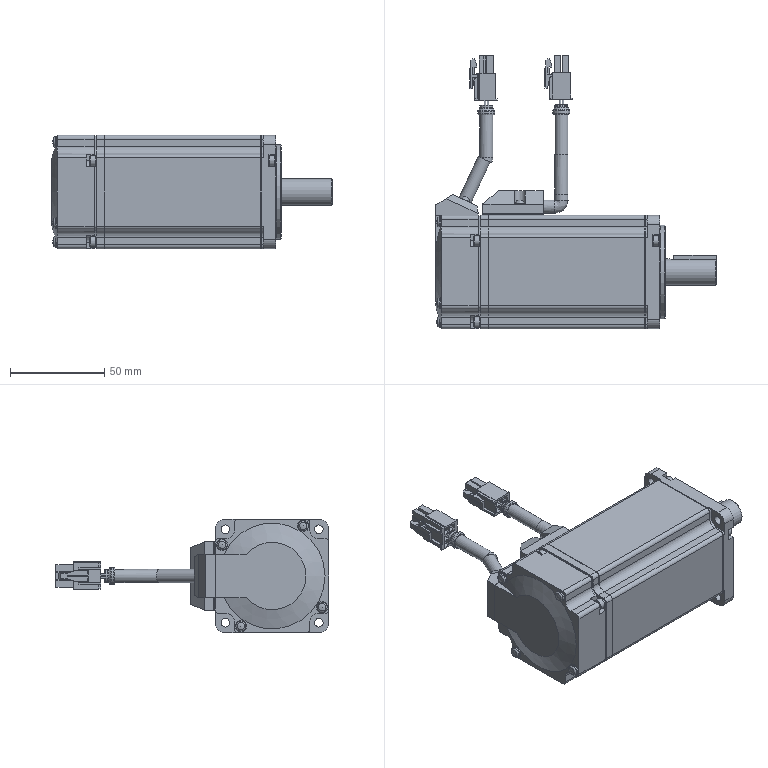Part | NX | 7 solids | 800 faces | box 148.5 x 144.8 x 60 mm | volume 412247 mm3 | plane 561 | cylinder 190 | cone 27 | spline 22 | commonest cylinder face diameters 4 x54 8 x28 0.6 x18 6 x14 1 x10 2.6 x10